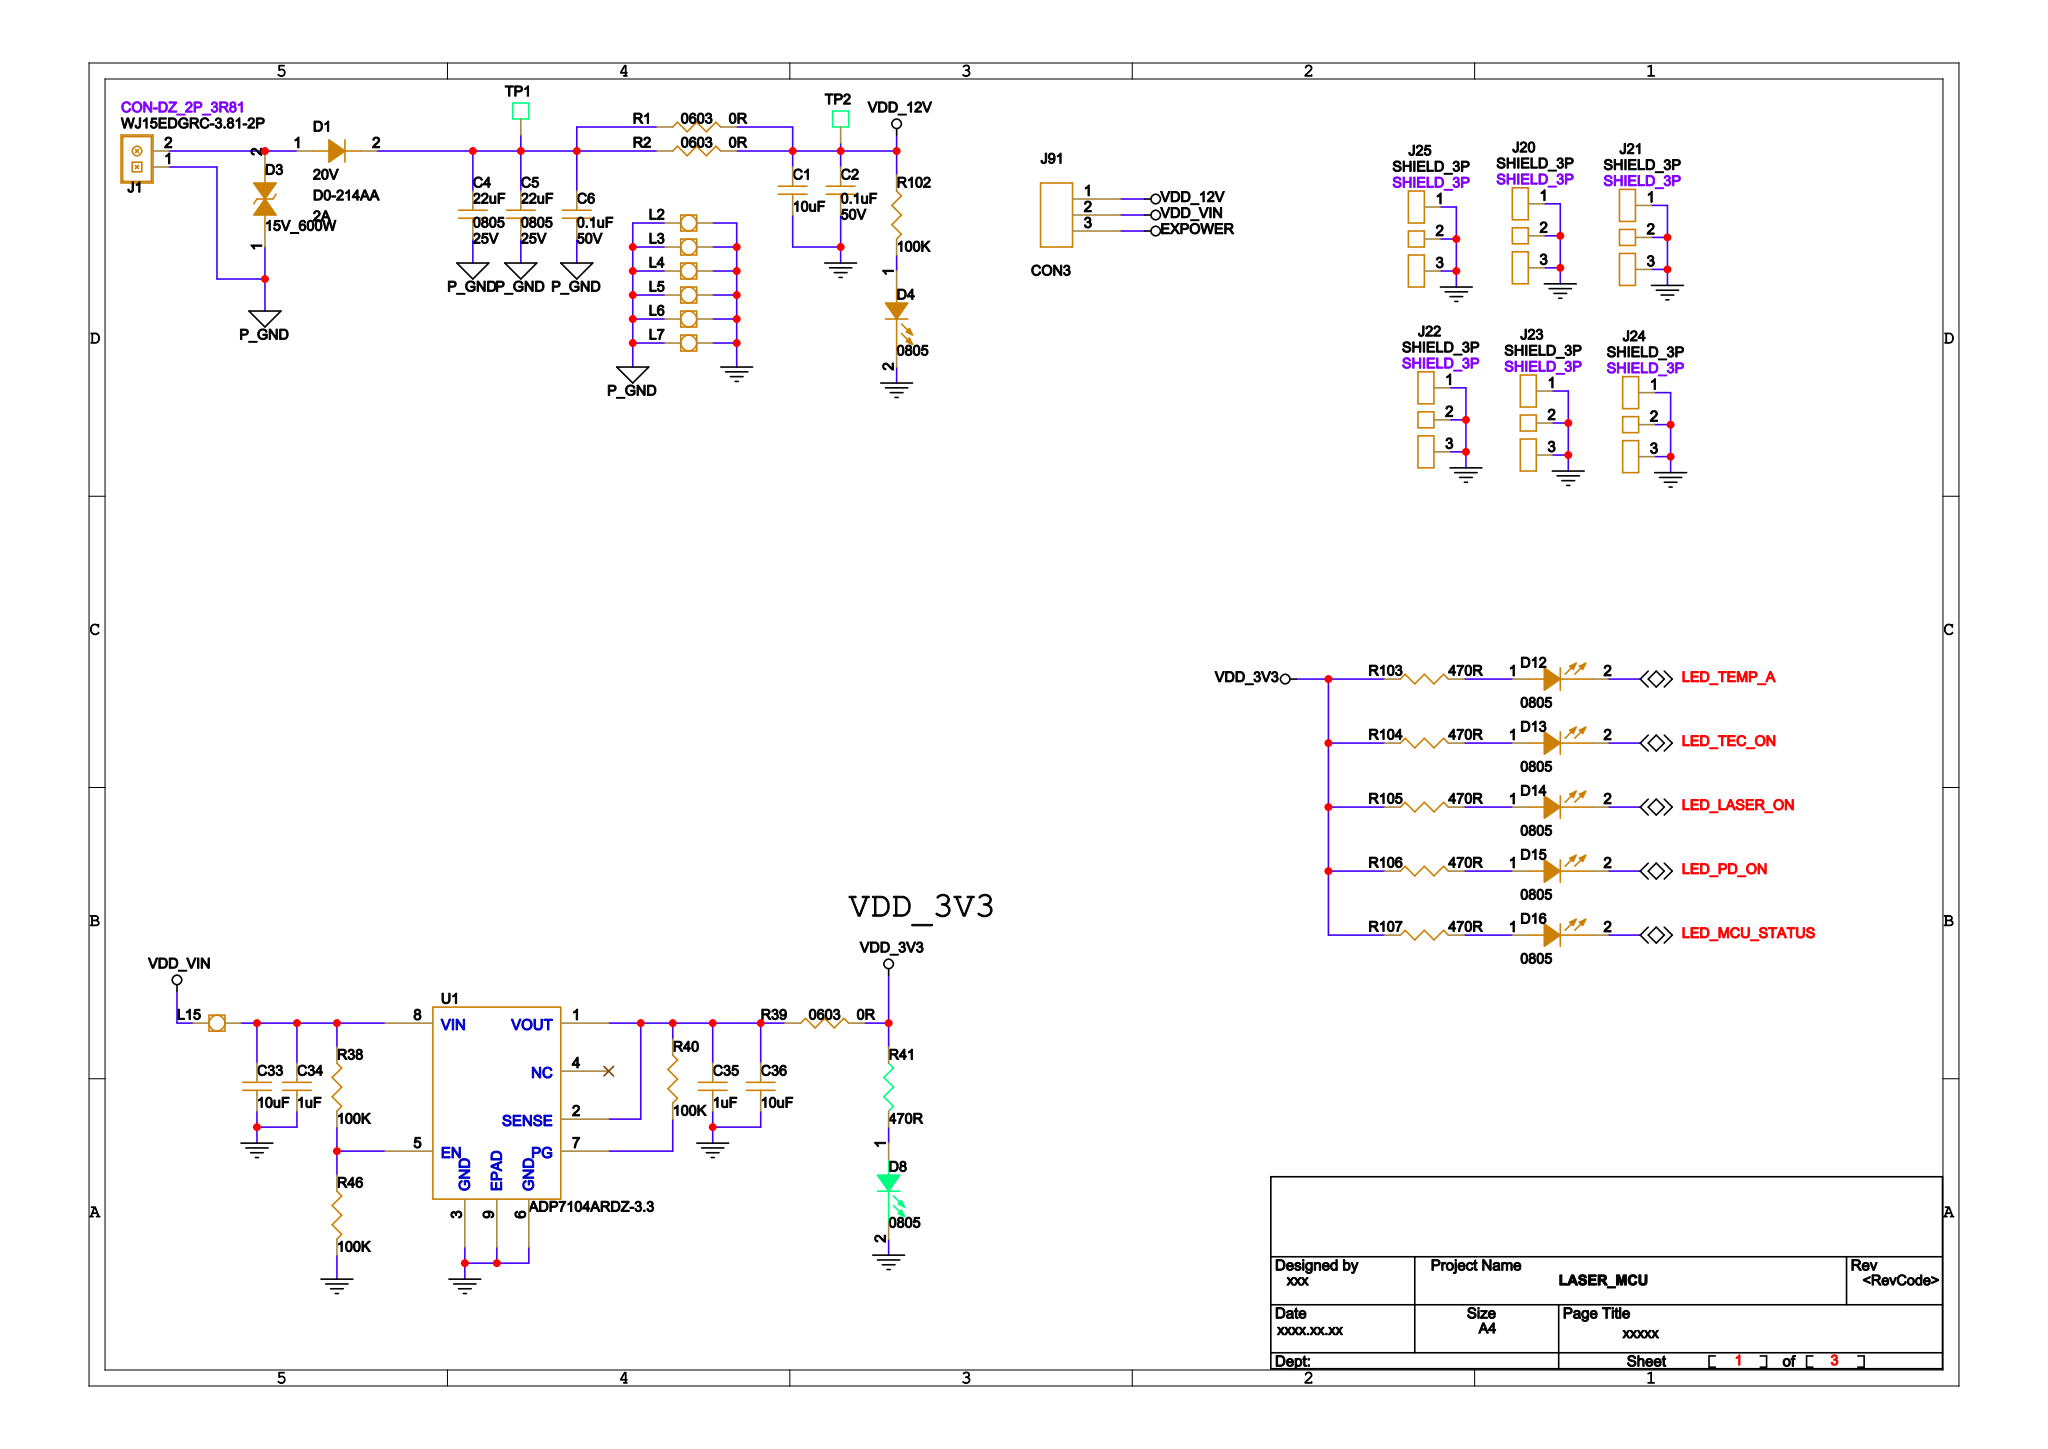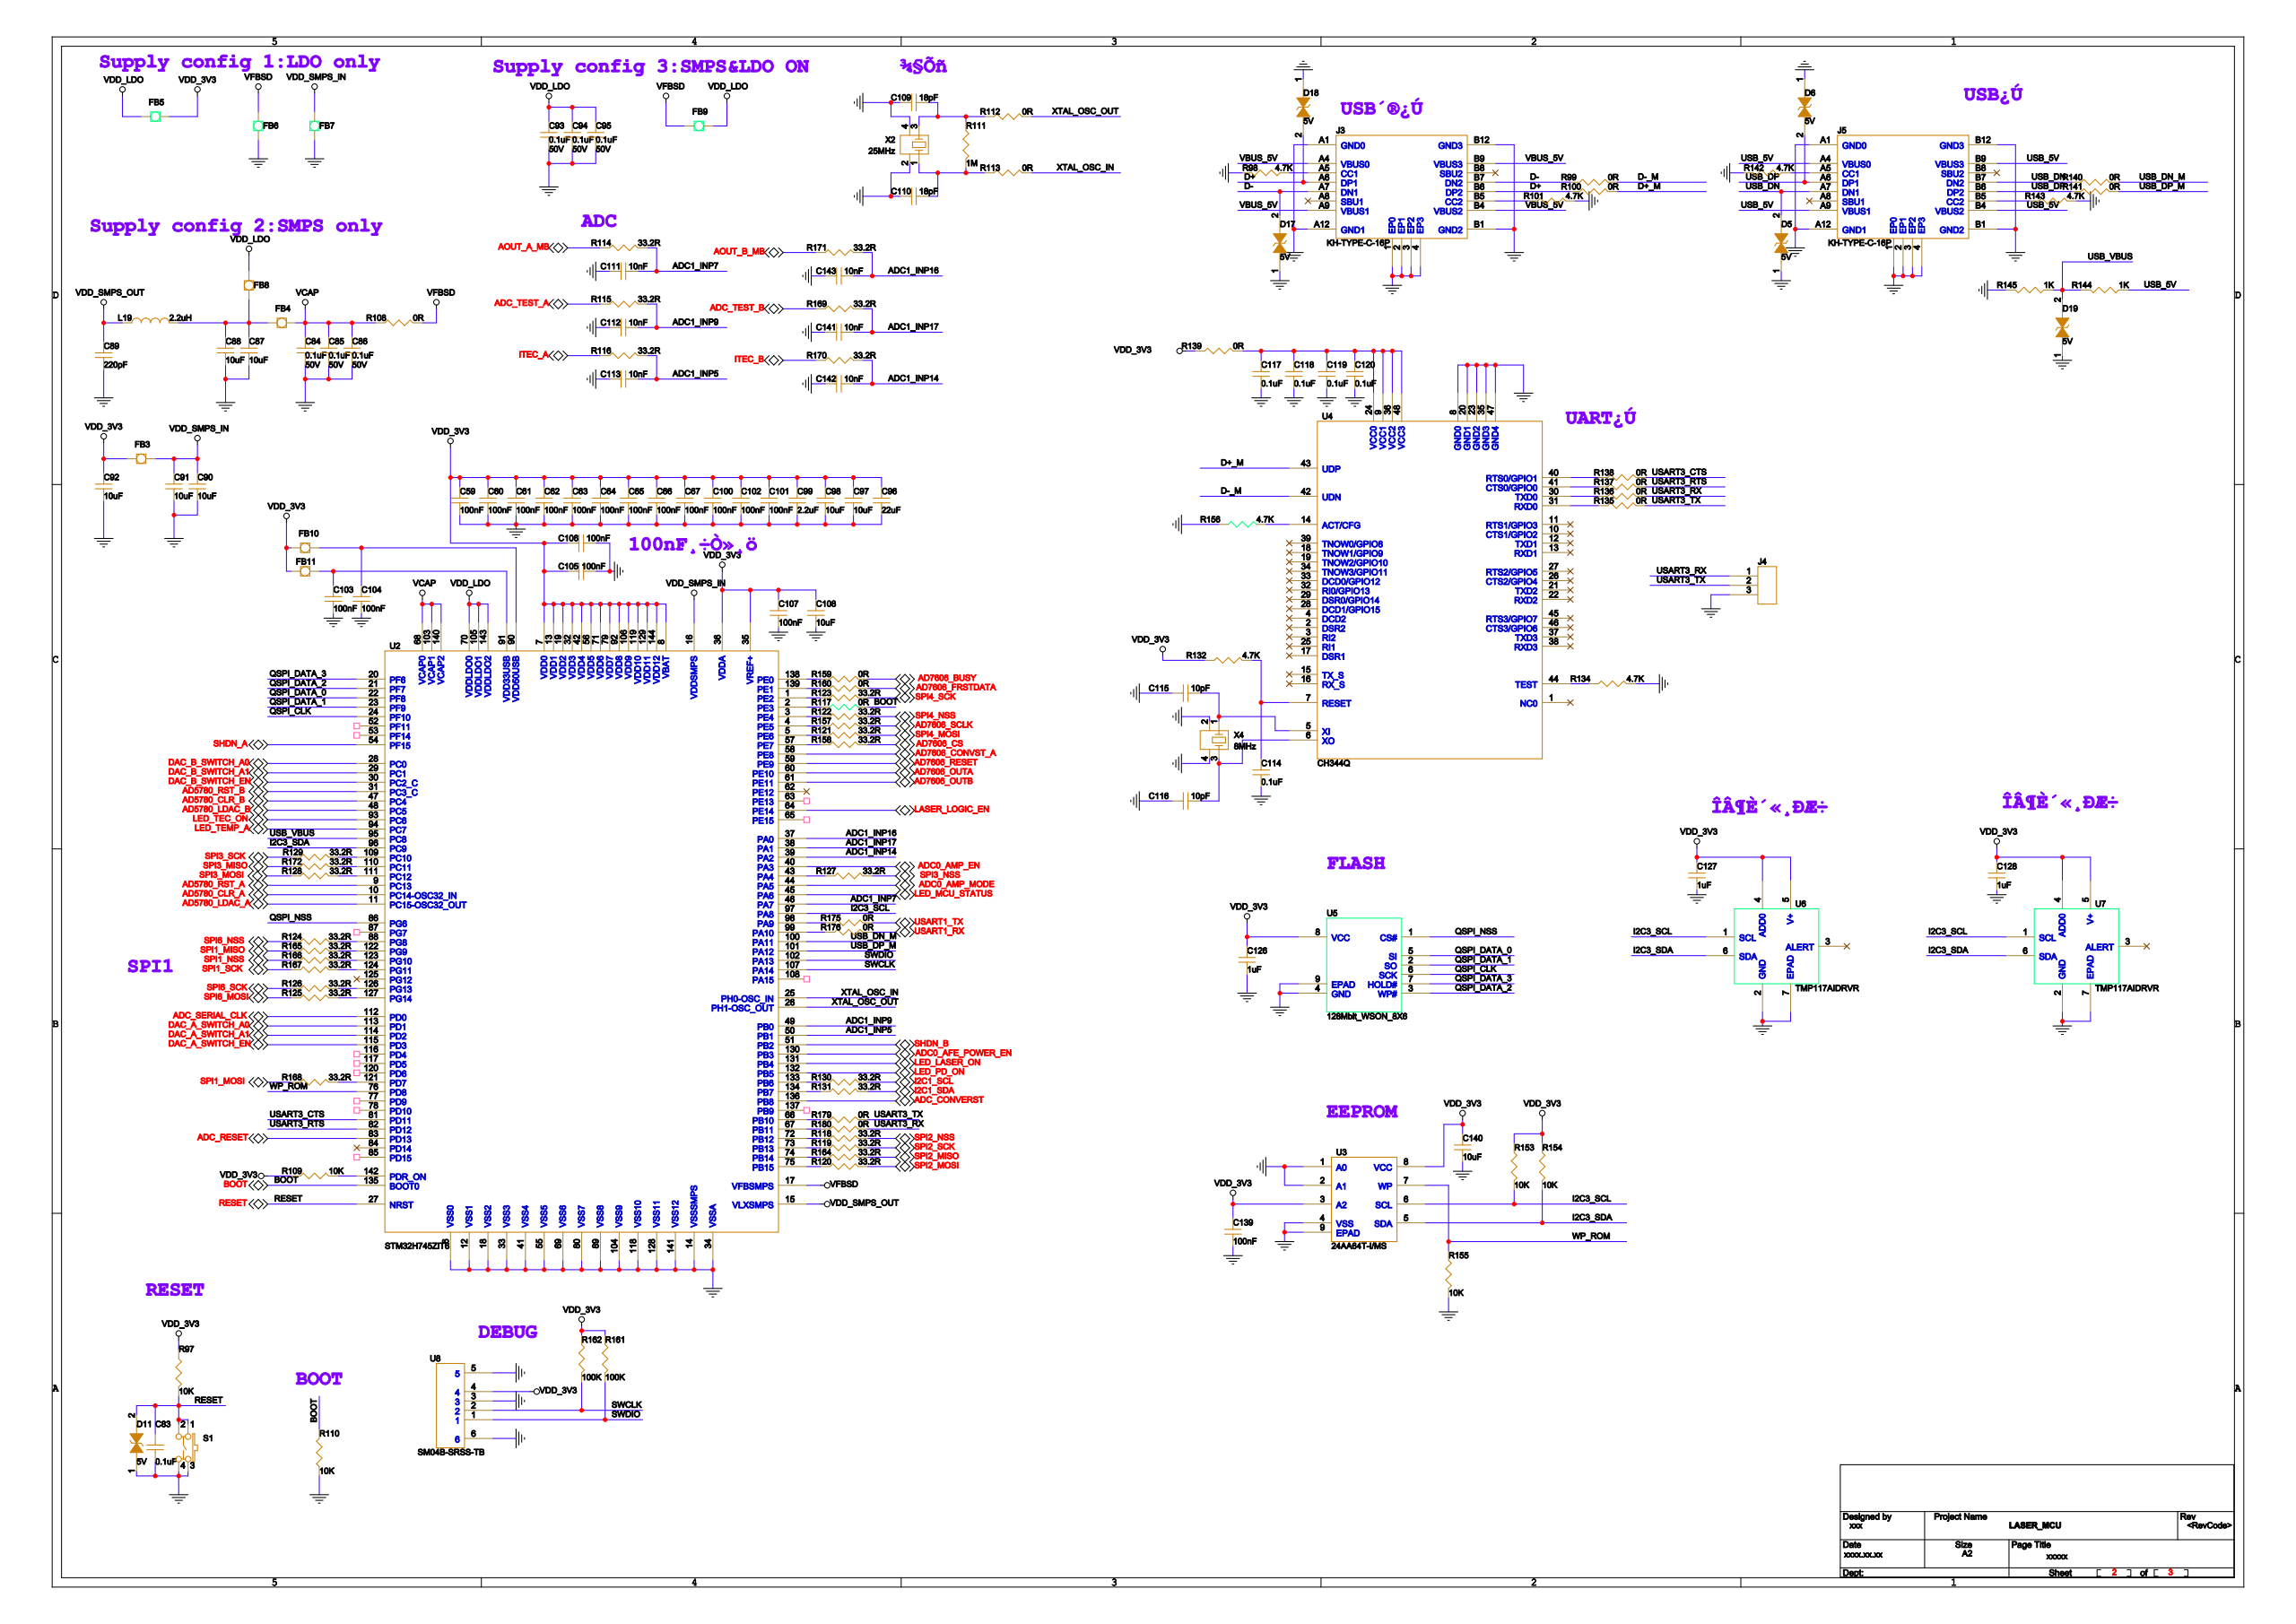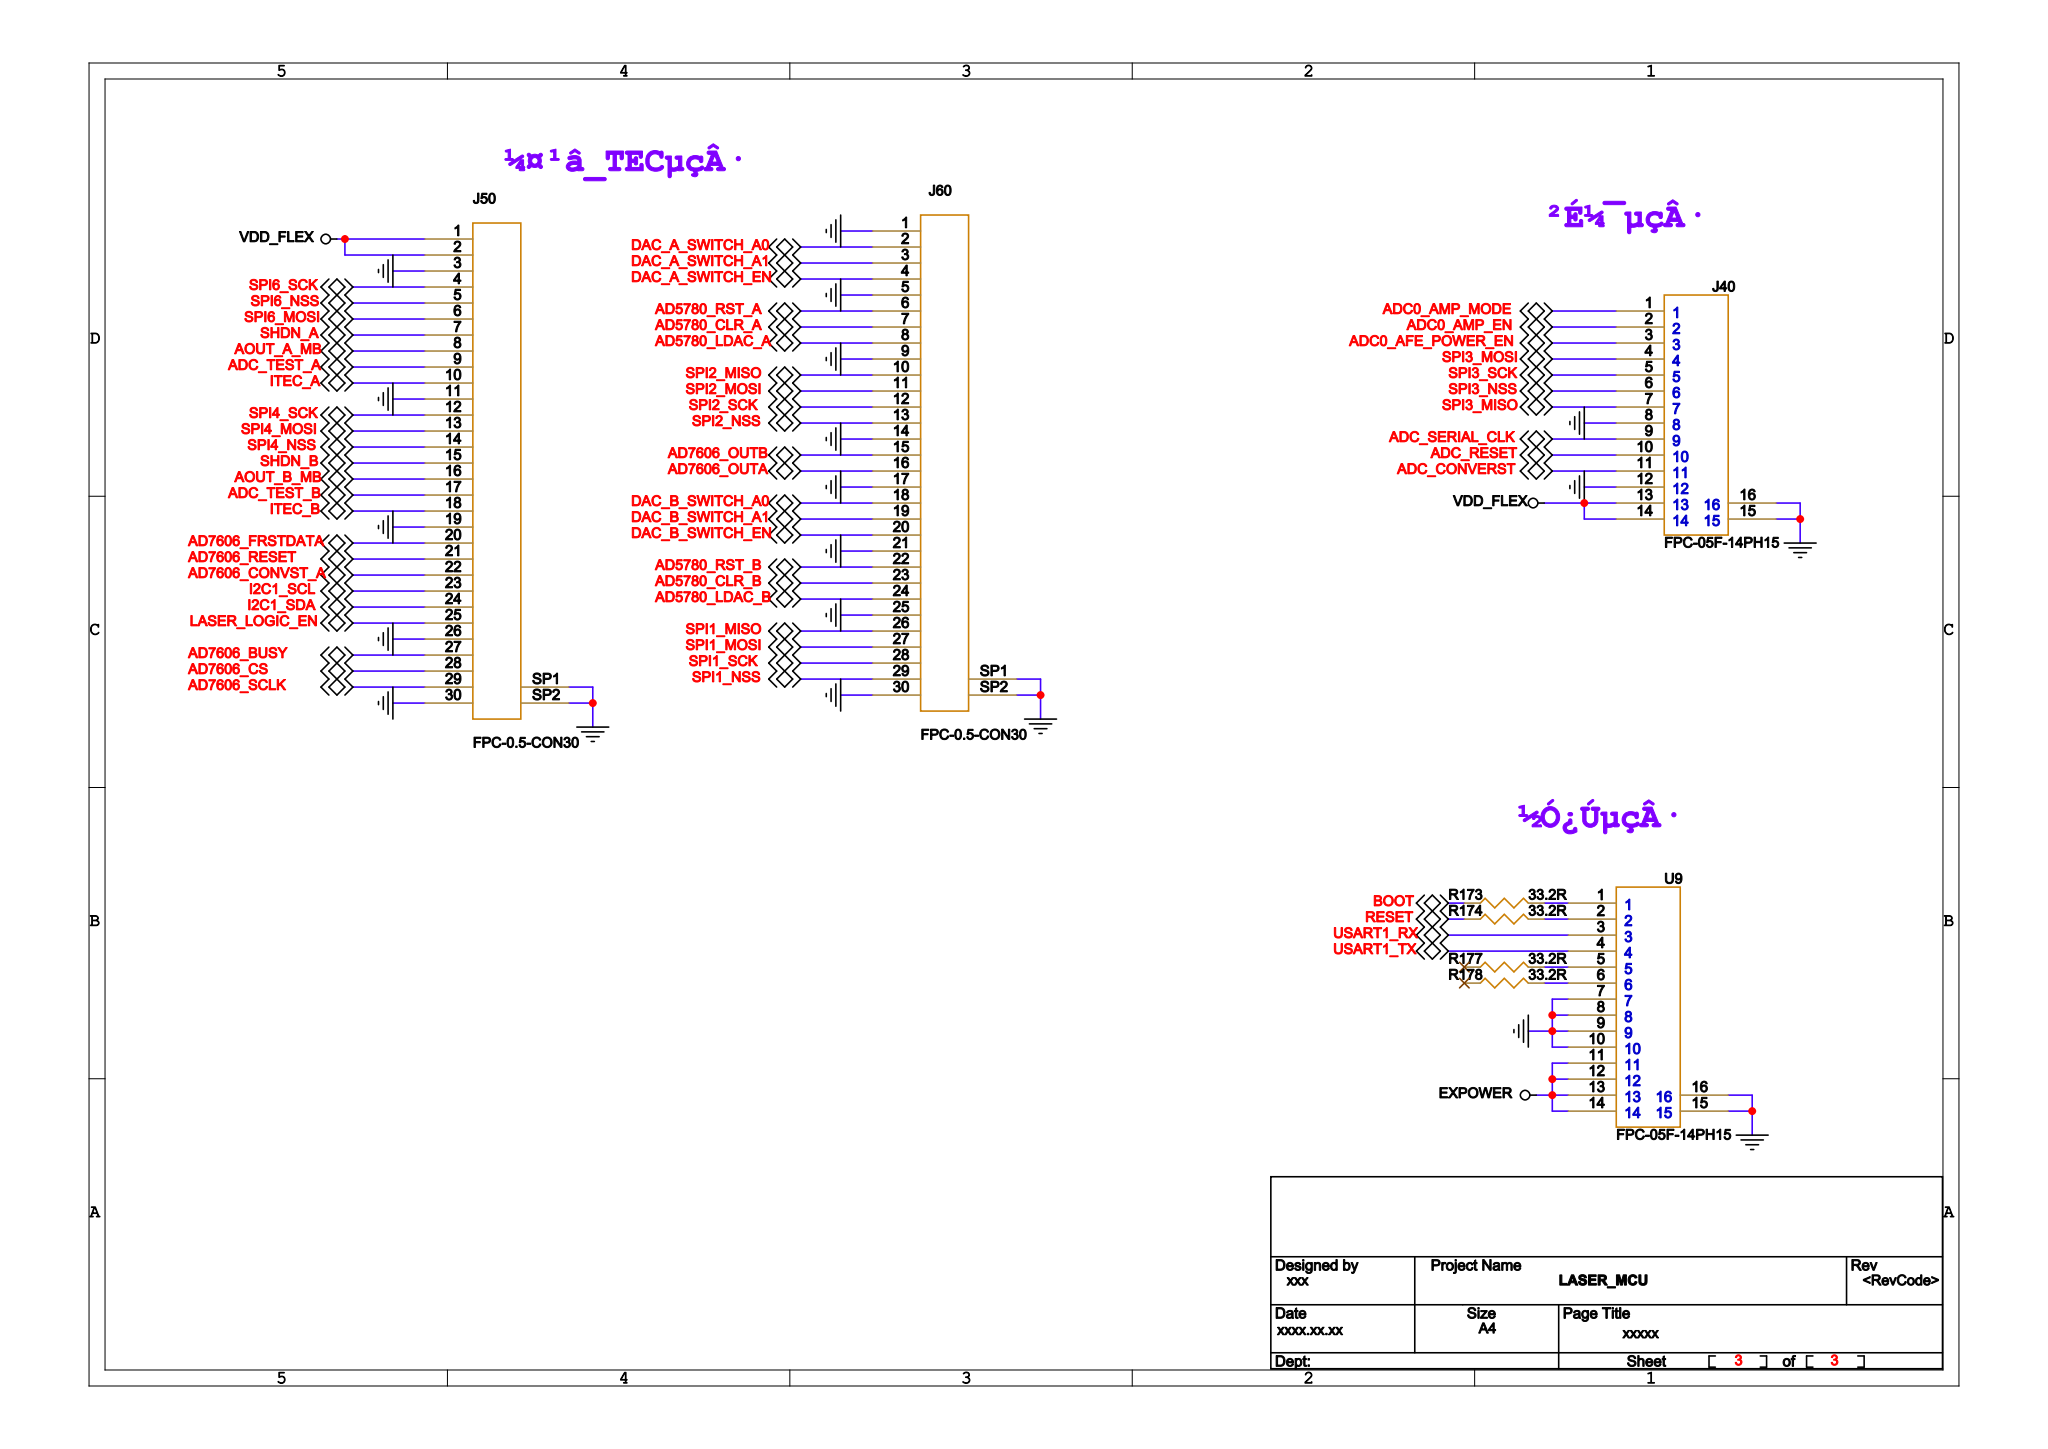Circuit board | Cadence Allegro | 206 parts | 176 nets
Bill of materials:
SYM_NAME,COMP_DEVICE_TYPE,COMP_VALUE,COMP_TOL,COMP_CLASS,REFDES
A185_C_1206_H160,CAP NP_A185_C_1206_H160_10UF_GR,10uF,,IC,C1
A183_C_0402_H50,CAP NP_A183_C_0402_H50_0.1UF_CC,0.1uF,,IC,C2
A186_C_0805_H125,CAP NP_A186_C_0805_H125_22UF_CL,22uF,,IC,C4
A186_C_0805_H125,CAP NP_A186_C_0805_H125_22UF_CL,22uF,,IC,C5
A183_C_0402_H50,CAP NP_A183_C_0402_H50_0.1UF_CC,0.1uF,,IC,C6
A185_C_1206_H160,CAP NP_A185_C_1206_H160_10UF_GR,10uF,,IC,C33
A183_C_0402_H50,CAP NP_A183_C_0402_H50_1UF_CL05,1uF,,IC,C34
A183_C_0402_H50,CAP NP_A183_C_0402_H50_1UF_CL05,1uF,,IC,C35
A185_C_1206_H160,CAP NP_A185_C_1206_H160_10UF_GR,10uF,,IC,C36
A183_C_0402_H50,CAP NP_A183_C_0402_H50_100NF_GR,100nF,,IC,C59
A183_C_0402_H50,CAP NP_A183_C_0402_H50_100NF_GR,100nF,,IC,C60
A183_C_0402_H50,CAP NP_A183_C_0402_H50_100NF_GR,100nF,,IC,C61
A183_C_0402_H50,CAP NP_A183_C_0402_H50_100NF_GR,100nF,,IC,C62
A183_C_0402_H50,CAP NP_A183_C_0402_H50_100NF_GR,100nF,,IC,C63
A183_C_0402_H50,CAP NP_A183_C_0402_H50_100NF_GR,100nF,,IC,C64
A183_C_0402_H50,CAP NP_A183_C_0402_H50_100NF_GR,100nF,,IC,C65
A183_C_0402_H50,CAP NP_A183_C_0402_H50_100NF_GR,100nF,,IC,C66
A183_C_0402_H50,CAP NP_A183_C_0402_H50_100NF_GR,100nF,,IC,C67
A454_C_0201_H33,CAP NP_A454_C_0201_H33_0.1UF _G,0.1uF,,IC,C83
A183_C_0402_H50,CAP NP_A183_C_0402_H50_0.1UF_CC,0.1uF,,IC,C84
A183_C_0402_H50,CAP NP_A183_C_0402_H50_0.1UF_CC,0.1uF,,IC,C85
A183_C_0402_H50,CAP NP_A183_C_0402_H50_0.1UF_CC,0.1uF,,IC,C86
A185_C_1206_H160,CAP NP_A185_C_1206_H160_10UF_GR,10uF,,IC,C87
A185_C_1206_H160,CAP NP_A185_C_1206_H160_10UF_GR,10uF,,IC,C88
A183_C_0402_H50,CAP NP_A183_C_0402_H50_220PF_GR,220pF,,IC,C89
A185_C_1206_H160,CAP NP_A185_C_1206_H160_10UF_GR,10uF,,IC,C90
A185_C_1206_H160,CAP NP_A185_C_1206_H160_10UF_GR,10uF,,IC,C91
A185_C_1206_H160,CAP NP_A185_C_1206_H160_10UF_GR,10uF,,IC,C92
A183_C_0402_H50,CAP NP_A183_C_0402_H50_0.1UF_CC,0.1uF,,IC,C93
A183_C_0402_H50,CAP NP_A183_C_0402_H50_0.1UF_CC,0.1uF,,IC,C94
A183_C_0402_H50,CAP NP_A183_C_0402_H50_0.1UF_CC,0.1uF,,IC,C95
A186_C_0805_H125,CAP NP_A186_C_0805_H125_22UF_GR,22uF,,IC,C96
A185_C_1206_H160,CAP NP_A185_C_1206_H160_10UF_GR,10uF,,IC,C97
A185_C_1206_H160,CAP NP_A185_C_1206_H160_10UF_GR,10uF,,IC,C98
A183_C_0402_H50,CAP NP_A183_C_0402_H50_2.2UF_GR,2.2uF,,IC,C99
A183_C_0402_H50,CAP NP_A183_C_0402_H50_100NF_GR,100nF,,IC,C100
A183_C_0402_H50,CAP NP_A183_C_0402_H50_100NF_GR,100nF,,IC,C101
A183_C_0402_H50,CAP NP_A183_C_0402_H50_100NF_GR,100nF,,IC,C102
A183_C_0402_H50,CAP NP_A183_C_0402_H50_100NF_GR,100nF,,IC,C103
A183_C_0402_H50,CAP NP_A183_C_0402_H50_100NF_GR,100nF,,IC,C104
A183_C_0402_H50,CAP NP_A183_C_0402_H50_100NF_GR,100nF,,IC,C105
A183_C_0402_H50,CAP NP_A183_C_0402_H50_100NF_GR,100nF,,IC,C106
A183_C_0402_H50,CAP NP_A183_C_0402_H50_100NF_GR,100nF,,IC,C107
A185_C_1206_H160,CAP NP_A185_C_1206_H160_10UF_GR,10uF,,IC,C108
A183_C_0402_H50,CAP NP_A183_C_0402_H50_18PF_GRM,18pF,,IC,C109
A183_C_0402_H50,CAP NP_A183_C_0402_H50_18PF_GRM,18pF,,IC,C110
A183_C_0402_H50,CAP NP_A183_C_0402_H50_10NF_GRM,10nF,,IC,C111
A183_C_0402_H50,CAP NP_A183_C_0402_H50_10NF_GRM,10nF,,IC,C112
A183_C_0402_H50,CAP NP_A183_C_0402_H50_10NF_GRM,10nF,,IC,C113
A183_C_0402_H50,CAP NP_A183_C_0402_H50_0.1UF_GR,0.1uF,,IC,C114
A183_C_0402_H50,CAP NP_A183_C_0402_H50_10PF_GRM,10pF,,IC,C115
A183_C_0402_H50,CAP NP_A183_C_0402_H50_10PF_GRM,10pF,,IC,C116
A183_C_0402_H50,CAP NP_A183_C_0402_H50_0.1UF_GR,0.1uF,,IC,C117
A183_C_0402_H50,CAP NP_A183_C_0402_H50_0.1UF_GR,0.1uF,,IC,C118
A183_C_0402_H50,CAP NP_A183_C_0402_H50_0.1UF_GR,0.1uF,,IC,C119
A183_C_0402_H50,CAP NP_A183_C_0402_H50_0.1UF_GR,0.1uF,,IC,C120
A183_C_0402_H50,CAP NP_A183_C_0402_H50_1UF_CL05,1uF,,IC,C126
A183_C_0402_H50,CAP NP_A183_C_0402_H50_1UF_CL05,1uF,,IC,C127
A183_C_0402_H50,CAP NP_A183_C_0402_H50_1UF_CL05,1uF,,IC,C128
A183_C_0402_H50,CAP NP_A183_C_0402_H50_100NF_GR,100nF,,IC,C139
A184_C_0603_H80,CAP NP_A184_C_0603_H80_10UF_GRM,10uF,,IC,C140
A183_C_0402_H50,CAP NP_A183_C_0402_H50_10NF_GRM,10nF,,IC,C141
A183_C_0402_H50,CAP NP_A183_C_0402_H50_10NF_GRM,10nF,,IC,C142
A183_C_0402_H50,CAP NP_A183_C_0402_H50_10NF_GRM,10nF,,IC,C143
DO_214AA_H244,DIODE_DO_214AA_H244_20V_SS22,20V,,IC,D1
A018_DO_214AA_H244,TVS_CA_A018_DO_214AA_H244_15V_6,15V_600W,,IC,D3
LED0805,LED_SINGLE_LED0805_LED_SINGLE_5,LED_SINGLE,,IC,D4
A179_D_0402,TVS_CA_A179_D_0402_5V_CG0402MLC,5V,,IC,D5
A179_D_0402,TVS_CA_A179_D_0402_5V_CG0402MLC,5V,,IC,D6
LED0805,LED_SINGLE_LED0805_LED_SINGLE_5,LED_SINGLE,,IC,D8
A179_D_0402,TVS_CA_A179_D_0402_5V_CG0402MLC,5V,,IC,D11
LED0805,LED_SINGLE_LED0805_LED_SINGLE_5,LED_SINGLE,,IC,D12
LED0805,LED_SINGLE_LED0805_LED_SINGLE_5,LED_SINGLE,,IC,D13
LED0805,LED_SINGLE_LED0805_LED_SINGLE_5,LED_SINGLE,,IC,D14
LED0805,LED_SINGLE_LED0805_LED_SINGLE_5,LED_SINGLE,,IC,D15
LED0805,LED_SINGLE_LED0805_LED_SINGLE_5,LED_SINGLE,,IC,D16
A179_D_0402,TVS_CA_A179_D_0402_5V_CG0402MLC,5V,,IC,D17
A179_D_0402,TVS_CA_A179_D_0402_5V_CG0402MLC,5V,,IC,D18
A179_D_0402,TVS_CA_A179_D_0402_5V_CG0402MLC,5V,,IC,D19
A041_L_0402_H60,BLM03PX800SN1_A041_L_0402_H60_B,BLM15EG121SN1D,,IC,FB3
A041_L_0402_H60,BLM03PX800SN1_A041_L_0402_H60_B,BLM15EG121SN1D,,IC,FB4
A041_L_0402_H60,BLM03PX800SN1_A041_L_0402_H60_B,BLM15EG121SN1D,,IC,FB5
A041_L_0402_H60,BLM03PX800SN1_A041_L_0402_H60_B,BLM15EG121SN1D,,IC,FB6
A041_L_0402_H60,BLM03PX800SN1_A041_L_0402_H60_B,BLM15EG121SN1D,,IC,FB7
A041_L_0402_H60,BLM03PX800SN1_A041_L_0402_H60_B,BLM15EG121SN1D,,IC,FB8
A041_L_0402_H60,BLM03PX800SN1_A041_L_0402_H60_B,BLM15EG121SN1D,,IC,FB9
A041_L_0402_H60,BLM03PX800SN1_A041_L_0402_H60_B,BLM15EG121SN1D,,IC,FB10
A041_L_0402_H60,BLM03PX800SN1_A041_L_0402_H60_B,BLM15EG121SN1D,,IC,FB11
CON-DZ_2P_3R81,CON-PIN HEADER_SINGLE_2P_CON-DZ,WJ15EDGRC-3.81-2P,,IC,J1
USB-4P-B,KH-TYPE-C-16P_USB-4P-B_KH-TYPE-,KH-TYPE-C-16P,,IC,J3
HEADER3,CON3_HEADER3_CON3_22-28-5034,CON3,,IC,J4
USB-4P-B,KH-TYPE-C-16P_USB-4P-B_KH-TYPE-,KH-TYPE-C-16P,,IC,J5
SHIELD_3P,SHIELD_3P_SHIELD_3P_SHIELD_3P,SHIELD_3P,,IC,J20
SHIELD_3P,SHIELD_3P_SHIELD_3P_SHIELD_3P,SHIELD_3P,,IC,J21
SHIELD_3P,SHIELD_3P_SHIELD_3P_SHIELD_3P,SHIELD_3P,,IC,J22
SHIELD_3P,SHIELD_3P_SHIELD_3P_SHIELD_3P,SHIELD_3P,,IC,J23
SHIELD_3P,SHIELD_3P_SHIELD_3P_SHIELD_3P,SHIELD_3P,,IC,J24
SHIELD_3P,SHIELD_3P_SHIELD_3P_SHIELD_3P,SHIELD_3P,,IC,J25
FPC-05F-14PH15,FPC-05F-14PH15_FPC-05F-14PH15_F,FPC-05F-14PH15,,IC,J40
FPCS_05PITCH_30P,FPC-0.5-CON30_FPCS_05PITCH_30P_,FPC-0.5-CON30,,IC,J50
FPCS_05PITCH_30P,FPC-0.5-CON30_FPCS_05PITCH_30P_,FPC-0.5-CON30,,IC,J60
HEADER3,CON3_HEADER3_CON3_22-28-5034,CON3,,IC,J91
A041_L_0402_H60,BEAD_A041_L_0402_H60_120OHM_100,120ohm_100MHz_1.5A,,IC,L2
A041_L_0402_H60,BEAD_A041_L_0402_H60_120OHM_100,120ohm_100MHz_1.5A,,IC,L3
A041_L_0402_H60,BEAD_A041_L_0402_H60_120OHM_100,120ohm_100MHz_1.5A,,IC,L4
A041_L_0402_H60,BEAD_A041_L_0402_H60_120OHM_100,120ohm_100MHz_1.5A,,IC,L5
A041_L_0402_H60,BEAD_A041_L_0402_H60_120OHM_100,120ohm_100MHz_1.5A,,IC,L6
A041_L_0402_H60,BEAD_A041_L_0402_H60_120OHM_100,120ohm_100MHz_1.5A,,IC,L7
A041_L_0402_H60,BEAD_A041_L_0402_H60_120OHM_100,120ohm_100MHz_1.5A,,IC,L15
A041_L_0402_RF_H60,INDUCTOR_A041_L_0402_RF_H60_2.2,2.2uH,,IC,L19
A082_R_0603_H45,R_A082_R_0603_H45_0R_0603WAF000,0R,,IC,R1
A082_R_0603_H45,R_A082_R_0603_H45_0R_0603WAF000,0R,,IC,R2
A081_R_0402_H35,R_A081_R_0402_H35_100K_RC0402FR,100K,,IC,R38
A082_R_0603_H45,R_A082_R_0603_H45_0R_0603WAF000,0R,,IC,R39
A081_R_0402_H35,R_A081_R_0402_H35_100K_RC0402FR,100K,,IC,R40
A081_R_0402_H35,R_A081_R_0402_H35_470R_0402WGJ0,470R,,IC,R41
A081_R_0402_H35,R_A081_R_0402_H35_100K_RC0402FR,100K,,IC,R46
A454_C_0201_H33,R_A454_C_0201_H33_10K_0201WMJ01,10K,,IC,R97
A081_R_0402_H35,R_A081_R_0402_H35_4.7K_0402WGJ0,4.7K,,IC,R98
A081_R_0402_H35,R_A081_R_0402_H35_0R_RC0402FR-0,0R,,DISCRETE,R99
A081_R_0402_H35,R_A081_R_0402_H35_0R_RC0402FR-0,0R,,DISCRETE,R100
A081_R_0402_H35,R_A081_R_0402_H35_4.7K_0402WGJ0,4.7K,,IC,R101
A081_R_0402_H35,R_A081_R_0402_H35_100K_RC0402FR,100K,,IC,R102
A081_R_0402_H35,R_A081_R_0402_H35_470R_0402WGJ0,470R,,IC,R103
A081_R_0402_H35,R_A081_R_0402_H35_470R_0402WGJ0,470R,,IC,R104
A081_R_0402_H35,R_A081_R_0402_H35_470R_0402WGJ0,470R,,IC,R105
A081_R_0402_H35,R_A081_R_0402_H35_470R_0402WGJ0,470R,,IC,R106
A081_R_0402_H35,R_A081_R_0402_H35_470R_0402WGJ0,470R,,IC,R107
A082_R_0603_H45,R_A082_R_0603_H45_0R_0603WAF000,0R,,IC,R108
A081_R_0402_H35,R_A081_R_0402_H35_10K_0402WGF10,10K,,IC,R109
A081_R_0402_H35,R_A081_R_0402_H35_10K_0402WGF10,10K,,IC,R110
A081_R_0402_H35,R_A081_R_0402_H35_1M_0402WGF100,1M,,IC,R111
A081_R_0402_H35,R_A081_R_0402_H35_0R_RC0402FR-0,0R,,DISCRETE,R112
A081_R_0402_H35,R_A081_R_0402_H35_0R_RC0402FR-0,0R,,DISCRETE,R113
A081_R_0402_H35,R_A081_R_0402_H35_33.2R_0402WGF,33.2R,,IC,R114
A081_R_0402_H35,R_A081_R_0402_H35_33.2R_0402WGF,33.2R,,IC,R115
A081_R_0402_H35,R_A081_R_0402_H35_33.2R_0402WGF,33.2R,,IC,R116
A081_R_0402_H35,R_A081_R_0402_H35_0R_RC0402FR-0,0R,,DISCRETE,R117
A081_R_0402_H35,R_A081_R_0402_H35_33.2R_0402WGF,33.2R,,IC,R118
A081_R_0402_H35,R_A081_R_0402_H35_33.2R_0402WGF,33.2R,,IC,R119
A081_R_0402_H35,R_A081_R_0402_H35_33.2R_0402WGF,33.2R,,IC,R120
A081_R_0402_H35,R_A081_R_0402_H35_33.2R_0402WGF,33.2R,,IC,R121
A081_R_0402_H35,R_A081_R_0402_H35_33.2R_0402WGF,33.2R,,IC,R122
A081_R_0402_H35,R_A081_R_0402_H35_33.2R_0402WGF,33.2R,,IC,R123
A081_R_0402_H35,R_A081_R_0402_H35_33.2R_0402WGF,33.2R,,IC,R124
A081_R_0402_H35,R_A081_R_0402_H35_33.2R_0402WGF,33.2R,,IC,R125
A081_R_0402_H35,R_A081_R_0402_H35_33.2R_0402WGF,33.2R,,IC,R126
A081_R_0402_H35,R_A081_R_0402_H35_33.2R_0402WGF,33.2R,,IC,R127
A081_R_0402_H35,R_A081_R_0402_H35_33.2R_0402WGF,33.2R,,IC,R128
A081_R_0402_H35,R_A081_R_0402_H35_33.2R_0402WGF,33.2R,,IC,R129
A081_R_0402_H35,R_A081_R_0402_H35_33.2R_0402WGF,33.2R,,IC,R130
A081_R_0402_H35,R_A081_R_0402_H35_33.2R_0402WGF,33.2R,,IC,R131
A081_R_0402_H35,R_A081_R_0402_H35_4.7K_0402WGJ0,4.7K,,IC,R132
A081_R_0402_H35,R_A081_R_0402_H35_4.7K_0402WGJ0,4.7K,,IC,R134
A081_R_0402_H35,R_A081_R_0402_H35_0R_RC0402FR-0,0R,,DISCRETE,R135
A081_R_0402_H35,R_A081_R_0402_H35_0R_RC0402FR-0,0R,,DISCRETE,R136
A081_R_0402_H35,R_A081_R_0402_H35_0R_RC0402FR-0,0R,,DISCRETE,R137
A081_R_0402_H35,R_A081_R_0402_H35_0R_RC0402FR-0,0R,,DISCRETE,R138
A081_R_0402_H35,R_A081_R_0402_H35_0R_RC0402FR-0,0R,,DISCRETE,R139
A081_R_0402_H35,R_A081_R_0402_H35_0R_RC0402FR-0,0R,,DISCRETE,R140
A081_R_0402_H35,R_A081_R_0402_H35_0R_RC0402FR-0,0R,,DISCRETE,R141
A081_R_0402_H35,R_A081_R_0402_H35_4.7K_0402WGJ0,4.7K,,IC,R142
A081_R_0402_H35,R_A081_R_0402_H35_4.7K_0402WGJ0,4.7K,,IC,R143
A081_R_0402_H35,R_A081_R_0402_H35_1K_0402WGF100,1K,,IC,R144
A081_R_0402_H35,R_A081_R_0402_H35_1K_0402WGF100,1K,,IC,R145
A081_R_0402_H35,R_A081_R_0402_H35_10K_0402WGF10,10K,,IC,R153
A081_R_0402_H35,R_A081_R_0402_H35_10K_0402WGF10,10K,,IC,R154
A081_R_0402_H35,R_A081_R_0402_H35_10K_0402WGF10,10K,,IC,R155
A081_R_0402_H35,R_A081_R_0402_H35_4.7K_0402WGJ0,4.7K,,IC,R156
A081_R_0402_H35,R_A081_R_0402_H35_33.2R_0402WGF,33.2R,,IC,R157
A081_R_0402_H35,R_A081_R_0402_H35_33.2R_0402WGF,33.2R,,IC,R158
A081_R_0402_H35,R_A081_R_0402_H35_0R_RC0402FR-0,0R,,DISCRETE,R159
A081_R_0402_H35,R_A081_R_0402_H35_0R_RC0402FR-0,0R,,DISCRETE,R160
A081_R_0402_H35,R_A081_R_0402_H35_100K_0402WGF1,100K,,IC,R161
A081_R_0402_H35,R_A081_R_0402_H35_100K_0402WGF1,100K,,IC,R162
A081_R_0402_H35,R_A081_R_0402_H35_33.2R_0402WGF,33.2R,,IC,R164
A081_R_0402_H35,R_A081_R_0402_H35_33.2R_0402WGF,33.2R,,IC,R165
A081_R_0402_H35,R_A081_R_0402_H35_33.2R_0402WGF,33.2R,,IC,R166
A081_R_0402_H35,R_A081_R_0402_H35_33.2R_0402WGF,33.2R,,IC,R167
A081_R_0402_H35,R_A081_R_0402_H35_33.2R_0402WGF,33.2R,,IC,R168
A081_R_0402_H35,R_A081_R_0402_H35_33.2R_0402WGF,33.2R,,IC,R169
A081_R_0402_H35,R_A081_R_0402_H35_33.2R_0402WGF,33.2R,,IC,R170
A081_R_0402_H35,R_A081_R_0402_H35_33.2R_0402WGF,33.2R,,IC,R171
A081_R_0402_H35,R_A081_R_0402_H35_33.2R_0402WGF,33.2R,,IC,R172
A081_R_0402_H35,R_A081_R_0402_H35_33.2R_0402WGF,33.2R,,IC,R173
A081_R_0402_H35,R_A081_R_0402_H35_33.2R_0402WGF,33.2R,,IC,R174
A081_R_0402_H35,R_A081_R_0402_H35_0R_RC0402FR-0,0R,,DISCRETE,R175
A081_R_0402_H35,R_A081_R_0402_H35_0R_RC0402FR-0,0R,,DISCRETE,R176
A081_R_0402_H35,R_A081_R_0402_H35_33.2R_0402WGF,33.2R,,IC,R177
A081_R_0402_H35,R_A081_R_0402_H35_33.2R_0402WGF,33.2R,,IC,R178
A081_R_0402_H35,R_A081_R_0402_H35_0R_RC0402FR-0,0R,,DISCRETE,R179
A081_R_0402_H35,R_A081_R_0402_H35_0R_RC0402FR-0,0R,,DISCRETE,R180
SW_4-2P15-4P2X3P2-2P5,SW PUSHBUTTON_4P_A_SW_4-2P15-4P,SW PUSHBUTTON_4P_A,,IC,S1
Z055_TPS_30C,TP_S_Z055_TPS_30C_SMD_HOLE_30C_,SMD_HOLE_30C,,IC,TP1
Z055_TPS_30C,TP_S_Z055_TPS_30C_SMD_HOLE_30C_,SMD_HOLE_30C,,IC,TP2
RD-8-2,ADP7104ARDZ-3.3_RD-8-2_ADP7104A,ADP7104ARDZ-3.3,,IC,U1
QFP144-20X20-NO_PAD,STM32H745ZIT6_QFP144-20X20-NO_P,STM32H745ZIT6,,IC,U2
DFN8_2X3X1P1,24AA64T-I/MS_DFN8_2X3X1P1_24AA6,24AA64T-I/MS,,IC,U3
LQFP48-900X900-H160,CH344Q_LQFP48-900X900-H160_CH34,CH344Q,,IC,U4
A122_VFDFPN8_T_S800X600_H85,SPIFLASH_WSON8_A122_VFDFPN8_T_S,128Mbit_WSON_8X6,,IC,U5
WSON6_2X2,TMP117AIDRVR_WSON6_2X2_TMP117AI,TMP117AIDRVR,,IC,U6
WSON6_2X2,TMP117AIDRVR_WSON6_2X2_TMP117AI,TMP117AIDRVR,,IC,U7
SM04B-SRSS-TB,SM04B-SRSS-TB_SM04B-SRSS-TB_SM0,SM04B-SRSS-TB,,IC,U8
FPC-05F-14PH15,FPC-05F-14PH15_FPC-05F-14PH15_F,FPC-05F-14PH15,,IC,U9
X3225,CRYSTAL_4P_X3225_25MHZ_E3SB25E0,25MHz,,IC,X2
X3225,CRYSTAL_4P_X3225_8MHZ_TAXM8M4RD,8MHz,,IC,X4
Netlist (net: part-pin ...):
SWDIO: R161-2 U2-102 U8-1
SWCLK: R162-2 U2-107 U8-2
GND: C1-2 C2-2 C33-2 C34-2 C35-2 C36-2 C59-2 C60-2 C61-2 C62-2 C63-2 C64-2 C65-2 C66-2 C67-2 C83-2 C84-2 C85-2 C86-2 C87-2 C88-2 C89-2 C90-2 C91-2 C92-2 C93-2 C94-2 C95-2 C96-2 C97-2 C98-2 C99-2 C100-2 C101-2 C102-2 C103-2 C104-2 C105-2 C106-2 C107-2 C108-2 C109-1 C110-1 C111-1 C112-1 C113-1 C114-2 C115-1 C116-1 C117-2 C118-2 C119-2 C120-2 C126-2 C127-2 C128-2 C139-2 C140-2 C141-1 C142-1 C143-1 D4-2 D5-1 D6-1 D8-2 D11-1 D17-1 D18-1 D19-1 FB6-2 FB7-2 J3-1 J3-2 J3-3 J3-4 J3-A1 J3-A12 J3-B1 J3-B12 J4-3 J5-1 J5-2 J5-3 J5-4 J5-A1 J5-A12 J5-B1 J5-B12 J20-1 J20-2 J20-3 J21-1 J21-2 J21-3 J22-1 J22-2 J22-3 J23-1 J23-2 J23-3 J24-1 J24-2 J24-3 J25-1 J25-2 J25-3 J40-8 J40-12 J40-15 J40-16 J50-3 J50-11 J50-19 J50-26 J50-30 J50-SP1 J50-SP2 J60-1 J60-5 J60-9 J60-14 J60-17 J60-21 J60-25 J60-30 J60-SP1 J60-SP2 L2-2 L3-2 L4-2 L5-2 L6-2 L7-2 R46-2 R98-2 R101-2 R110-1 R134-2 R142-2 R143-2 R145-2 R155-2 R156-1 S1-3 S1-4 U1-3 U1-6 U1-9 U2-6 U2-12 U2-14 U2-18 U2-33 U2-34 U2-41 U2-55 U2-69 U2-80 U2-89 U2-104 U2-118 U2-128 U2-141 U3-1 U3-2 U3-4 U3-9 U4-8 U4-20 U4-23 U4-35 U4-47 U5-4 U5-9 U6-2 U6-7 U7-2 U7-7 U8-3 U8-5 U8-6 U9-7 U9-8 U9-9 U9-10 U9-15 U9-16 X2-2 X2-4 X4-2 X4-4
VDD_3V3: C59-1 C60-1 C61-1 C62-1 C63-1 C64-1 C65-1 C66-1 C67-1 C92-1 C96-1 C97-1 C98-1 C99-1 C100-1 C101-1 C102-1 C105-1 C106-1 C107-1 C108-1 C126-1 C127-1 C128-1 C139-1 C140-1 FB3-2 FB5-1 FB10-2 FB11-2 R39-2 R41-1 R97-2 R103-1 R104-1 R105-1 R106-1 R107-1 R109-1 R132-1 R139-1 R153-1 R154-1 R161-1 R162-1 U2-7 U2-8 U2-13 U2-19 U2-32 U2-35 U2-36 U2-42 U2-56 U2-71 U2-79 U2-92 U2-106 U2-119 U2-129 U2-144 U3-3 U3-8 U5-8 U6-4 U6-5 U7-4 U7-5 U8-4
I2C3_SCL: R153-2 U2-97 U3-6 U6-1 U7-1
I2C3_SDA: R154-2 U2-96 U3-5 U6-6 U7-6
BOOT: R110-2 R117-2 R173-1 U2-135
RESET: C83-1 D11-2 R97-1 R174-1 S1-1 S1-2 U2-27
ADC1_INP16: C143-2 R171-2 U2-37
ADC1_INP17: C141-2 R169-2 U2-38
N3324387: R176-1 U2-99
USB_DN_M: R140-2 U2-100
USB_DP_M: R141-2 U2-101
ADC1_INP14: C142-2 R170-2 U2-39
ADC0_AMP_EN: J40-2 U2-40
N3145912: R127-2 U2-43
ADC0_AMP_MODE: J40-1 U2-44
LED_MCU_STATUS: D16-2 U2-45
ADC1_INP7: C111-2 R114-2 U2-46
N3324383: R175-1 U2-98
ADC1_INP9: C112-2 R115-2 U2-49
ADC1_INP5: C113-2 R116-2 U2-50
N3332918: R179-1 U2-66
N3332968: R180-1 U2-67
N3143562: R118-1 U2-72
N3143554: R119-1 U2-73
N3282436: R164-1 U2-74
N3140912: R120-1 U2-75
SHDN_B: J50-15 U2-51
ADC0_AFE_POWER_EN: J40-3 U2-130
LED_LASER_ON: D14-2 U2-131
LED_PD_ON: D15-2 U2-132
N3147373: R130-1 U2-133
N3147369: R131-1 U2-134
ADC_CONVERST: J40-11 U2-136
DAC_B_SWITCH_A0: J60-18 U2-28
DAC_B_SWITCH_A1: J60-19 U2-29
N3146741: R129-2 U2-109
N3306667: R172-2 U2-110
N3309181: R128-2 U2-111
AD5780_RST_A: J60-6 U2-9
AD5780_CLR_A: J60-7 U2-10
AD5780_LDAC_A: J60-8 U2-11
DAC_B_SWITCH_EN: J60-20 U2-30
AD5780_RST_B: J60-22 U2-31
AD5780_CLR_B: J60-23 U2-47
AD5780_LDAC_B: J60-24 U2-48
LED_TEC_ON: D13-2 U2-93
LED_TEMP_A: D12-2 U2-94
USB_VBUS: D19-2 R144-2 R145-1 U2-95
ADC_SERIAL_CLK: J40-9 U2-112
DAC_A_SWITCH_A0: J60-2 U2-113
USART3_CTS: R138-2 U2-81
USART3_RTS: R137-2 U2-82
ADC_RESET: J40-10 U2-83
DAC_A_SWITCH_A1: J60-3 U2-114
DAC_A_SWITCH_EN: J60-4 U2-115
N3282701: R168-2 U2-121
WP_ROM: R155-1 U2-76 U3-7
N3119401: R109-2 U2-142
N3250496: R159-1 U2-138
N3250500: R160-1 U2-139
AD7606_OUTA: J60-16 U2-60
AD7606_OUTB: J60-15 U2-61
LASER_LOGIC_EN: J50-25 U2-64
N3137780: R123-1 U2-1
N3137774: R117-1 U2-2
N3137816: R122-1 U2-3
N3247877: R157-2 U2-4
N3137840: R121-1 U2-5
N3247871: R158-2 U2-57
AD7606_CONVST_A: J50-22 U2-58
AD7606_RESET: J50-21 U2-59
QSPI_CLK: U2-24 U5-6
SHDN_A: J50-7 U2-54
QSPI_DATA_3: U2-20 U5-7
QSPI_DATA_2: U2-21 U5-3
QSPI_DATA_0: U2-22 U5-5
QSPI_DATA_1: U2-23 U5-2
N3282581: R166-2 U2-123
N3282631: R167-2 U2-124
N3145078: R126-2 U2-126
N3145026: R125-2 U2-127
QSPI_NSS: U2-86 U5-1
N3144974: R124-2 U2-88
N3282529: R165-2 U2-122
XTAL_OSC_IN: R113-2 U2-25
XTAL_OSC_OUT: R112-2 U2-26
VCAP: C84-1 C85-1 C86-1 FB4-1 R108-1 U2-68 U2-103 U2-140
N3104381: C103-1 FB11-1 U2-91
N3105105: C104-1 FB10-1 U2-90
VDD_LDO: C93-1 C94-1 C95-1 FB5-2 FB8-1 FB9-1 U2-70 U2-105 U2-143
VDD_SMPS_IN: C90-1 C91-1 FB3-1 FB7-1 U2-16
VFBSD: FB6-1 FB9-2 R108-2 U2-17
VDD_SMPS_OUT: C89-1 L19-1 U2-15
VDD_FLEX: J40-13 J40-14 J50-1 J50-2
SPI3_MOSI: J40-4 R128-1
SPI3_SCK: J40-5 R129-1
SPI3_NSS: J40-6 R127-1
SPI3_MISO: J40-7 R172-1
N3322867: R173-2 U9-1
EXPOWER: J91-3 U9-11 U9-12 U9-13 U9-14
N3322871: R174-2 U9-2
USART1_RX: R176-2 U9-3
USART1_TX: R175-2 U9-4
N3332713: R177-2 U9-5
N3332717: R178-2 U9-6
N3122601: C109-2 R111-1 R112-1 X2-3
N3122593: C110-2 R111-2 R113-1 X2-1
N3154145: C114-1 R132-2 U4-7
N3154541: C117-1 C118-1 C119-1 C120-1 R139-2 U4-9 U4-24 U4-36 U4-48
N3154193: C115-2 U4-5 X4-1
N3154205: C116-2 U4-6 X4-3
D-: D17-2 J3-A7 J3-B7 R99-1
D+: D18-2 J3-A6 J3-B6 R100-1
USB_DN: D5-2 J5-A7 J5-B7 R140-1
USB_DP: D6-2 J5-A6 J5-B6 R141-1
N3084294: C87-1 C88-1 FB4-2 FB8-2 L19-2
N2484146: J3-A5 R98-1
N2485742: J3-B5 R101-1
VBUS_5V: J3-A4 J3-A9 J3-B4 J3-B9
N3180554: J5-A5 R142-1
N3180318: J5-B5 R143-1
USB_5V: J5-A4 J5-A9 J5-B4 J5-B9 R144-1
N3154485: R134-1 U4-44
N3243247: R156-2 U4-14
AOUT_A_MB: J50-8 R114-1
ADC_TEST_A: J50-9 R115-1
ITEC_A: J50-10 R116-1
SPI2_NSS: J60-13 R118-2
SPI2_SCK: J60-12 R119-2
SPI2_MOSI: J60-11 R120-2
SPI4_MOSI: J50-13 R121-2
SPI4_NSS: J50-14 R122-2
SPI4_SCK: J50-12 R123-2
SPI6_NSS: J50-5 R124-1
SPI6_MOSI: J50-6 R125-1
SPI6_SCK: J50-4 R126-1
I2C1_SCL: J50-23 R130-2
I2C1_SDA: J50-24 R131-2
AD7606_SCLK: J50-29 R157-1
AD7606_CS: J50-28 R158-1
SPI2_MISO: J60-10 R164-2
SPI1_MISO: J60-26 R165-1
SPI1_NSS: J60-29 R166-1
SPI1_SCK: J60-28 R167-1
SPI1_MOSI: J60-27 R168-1
ADC_TEST_B: J50-17 R169-1
ITEC_B: J50-18 R170-1
AOUT_B_MB: J50-16 R171-1
N2682318: R38-2 R46-1 U1-5
N2682514: R40-2 U1-7
N2682410: C35-1 C36-1 R39-1 R40-1 U1-1 U1-2
N2681860: C33-1 C34-1 L15-2 R38-1 U1-8
N3154333: R137-1 U4-41
N3154329: R138-1 U4-40
N3154453: R135-1 U4-31
N3154457: R136-1 U4-30
D-_M: R99-2 U4-42
D+_M: R100-2 U4-43
VDD_12V: C1-1 C2-1 J91-1 R1-2 R2-2 R102-1 TP2-1
N2682798: C4-1 C5-1 C6-1 D1-2 R1-1 R2-1 TP1-1
P_GND: C4-2 C5-2 C6-2 D3-1 J1-1 L2-1 L3-1 L4-1 L5-1 L6-1 L7-1
N2683254: D1-1 D3-2 J1-2
N2986746: D12-1 R103-2
N2988902: D13-1 R104-2
N2989028: D14-1 R105-2
N2989160: D15-1 R106-2
N2989295: D16-1 R107-2
N2683586: D4-1 R102-2
N2681952: D8-1 R41-2
AD7606_FRSTDATA: J50-20 R160-2
AD7606_BUSY: J50-27 R159-2
USART3_RX: J4-1 R136-2 R180-2
USART3_TX: J4-2 R135-2 R179-2
VDD_VIN: J91-2 L15-1